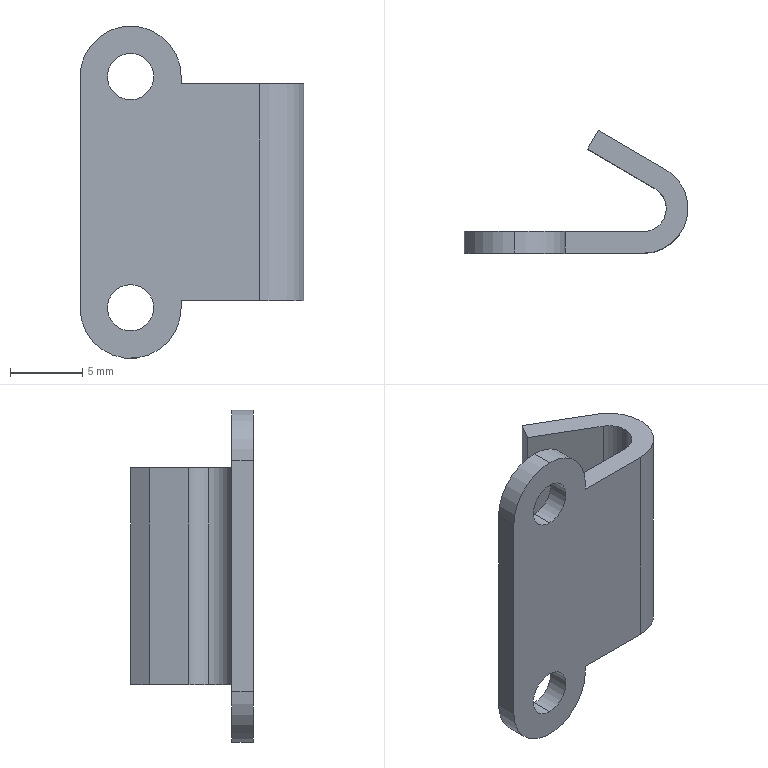Part | SolidWorks | features BaseBody 1 | 1 solid | 22 faces | box 15.5 x 8.5 x 23 mm | volume 582.779 mm3 | cylinder 11 | plane 11 | commonest cylinder face diameters 3.2 x6 7 x3 6.2 x2
STEP:
#1=CARTESIAN_POINT('',(-12.4,-3.1,8.));
#2=VERTEX_POINT('',#1);
#3=CARTESIAN_POINT('',(-8.9,-3.1,11.5));
#4=VERTEX_POINT('',#3);
#5=CARTESIAN_POINT('',(-8.9,-3.1,8.));
#6=DIRECTION('',(0.,1.,0.));
#7=DIRECTION('',(0.,0.,1.));
#8=AXIS2_PLACEMENT_3D('',#5,#6,#7);
#9=CIRCLE('',#8,3.5);
#10=EDGE_CURVE('',#2,#4,#9,.T.);
#11=ORIENTED_EDGE('',*,*,#10,.T.);
#12=CARTESIAN_POINT('',(-8.9,-1.6,11.5));
#13=VERTEX_POINT('',#12);
#14=CARTESIAN_POINT('',(-8.9,20.,11.5));
#15=DIRECTION('',(0.,1.,0.));
#16=VECTOR('',#15,1000.);
#17=LINE('',#14,#16);
#18=EDGE_CURVE('',#4,#13,#17,.T.);
#19=ORIENTED_EDGE('',*,*,#18,.T.);
#20=CARTESIAN_POINT('',(-12.4,-1.6,8.));
#21=VERTEX_POINT('',#20);
#22=CARTESIAN_POINT('',(-8.9,-1.6,8.));
#23=DIRECTION('',(0.,-1.,0.));
#24=DIRECTION('',(0.,0.,1.));
#25=AXIS2_PLACEMENT_3D('',#22,#23,#24);
#26=CIRCLE('',#25,3.5);
#27=EDGE_CURVE('',#13,#21,#26,.T.);
#28=ORIENTED_EDGE('',*,*,#27,.T.);
#29=CARTESIAN_POINT('',(-12.4,-1.6,8.));
#30=DIRECTION('',(0.,-1.,0.));
#31=VECTOR('',#30,1000.);
#32=LINE('',#29,#31);
#33=EDGE_CURVE('',#21,#2,#32,.T.);
#34=ORIENTED_EDGE('',*,*,#33,.T.);
#35=EDGE_LOOP('',(#11,#19,#28,#34));
#36=FACE_OUTER_BOUND('',#35,.T.);
#37=CARTESIAN_POINT('',(-8.9,20.,8.));
#38=DIRECTION('',(0.,1.,0.));
#39=DIRECTION('',(0.,0.,1.));
#40=AXIS2_PLACEMENT_3D('',#37,#38,#39);
#41=CYLINDRICAL_SURFACE('',#40,3.5);
#42=ADVANCED_FACE('',(#36),#41,.T.);
#43=CARTESIAN_POINT('',(-8.9,-3.1,-6.4));
#44=VERTEX_POINT('',#43);
#45=CARTESIAN_POINT('',(-8.9,-3.1,-9.6));
#46=VERTEX_POINT('',#45);
#47=CARTESIAN_POINT('',(-8.9,-3.1,-8.));
#48=DIRECTION('',(0.,-1.,0.));
#49=DIRECTION('',(0.,0.,1.));
#50=AXIS2_PLACEMENT_3D('',#47,#48,#49);
#51=CIRCLE('',#50,1.6);
#52=EDGE_CURVE('',#44,#46,#51,.T.);
#53=ORIENTED_EDGE('',*,*,#52,.T.);
#54=CARTESIAN_POINT('',(-8.9,-1.6,-9.6));
#55=VERTEX_POINT('',#54);
#56=CARTESIAN_POINT('',(-8.9,20.,-9.6));
#57=DIRECTION('',(0.,1.,0.));
#58=VECTOR('',#57,1000.);
#59=LINE('',#56,#58);
#60=EDGE_CURVE('',#46,#55,#59,.T.);
#61=ORIENTED_EDGE('',*,*,#60,.T.);
#62=CARTESIAN_POINT('',(-8.9,-1.6,-6.4));
#63=VERTEX_POINT('',#62);
#64=CARTESIAN_POINT('',(-8.9,-1.6,-8.));
#65=DIRECTION('',(0.,-1.,0.));
#66=DIRECTION('',(0.,0.,1.));
#67=AXIS2_PLACEMENT_3D('',#64,#65,#66);
#68=CIRCLE('',#67,1.6);
#69=EDGE_CURVE('',#63,#55,#68,.T.);
#70=ORIENTED_EDGE('',*,*,#69,.F.);
#71=CARTESIAN_POINT('',(-8.9,20.,-6.4));
#72=DIRECTION('',(0.,1.,0.));
#73=VECTOR('',#72,1000.);
#74=LINE('',#71,#73);
#75=EDGE_CURVE('',#44,#63,#74,.T.);
#76=ORIENTED_EDGE('',*,*,#75,.F.);
#77=EDGE_LOOP('',(#53,#61,#70,#76));
#78=FACE_OUTER_BOUND('',#77,.T.);
#79=CARTESIAN_POINT('',(-8.9,20.,-8.));
#80=DIRECTION('',(0.,1.,0.));
#81=DIRECTION('',(0.,0.,1.));
#82=AXIS2_PLACEMENT_3D('',#79,#80,#81);
#83=CYLINDRICAL_SURFACE('',#82,1.6);
#84=ADVANCED_FACE('',(#78),#83,.F.);
#85=CARTESIAN_POINT('',(-8.9,-3.1,9.6));
#86=VERTEX_POINT('',#85);
#87=CARTESIAN_POINT('',(-8.9,-3.1,6.4));
#88=VERTEX_POINT('',#87);
#89=CARTESIAN_POINT('',(-8.9,-3.1,8.));
#90=DIRECTION('',(0.,-1.,0.));
#91=DIRECTION('',(0.,0.,1.));
#92=AXIS2_PLACEMENT_3D('',#89,#90,#91);
#93=CIRCLE('',#92,1.6);
#94=EDGE_CURVE('',#86,#88,#93,.T.);
#95=ORIENTED_EDGE('',*,*,#94,.T.);
#96=CARTESIAN_POINT('',(-8.9,-1.6,6.4));
#97=VERTEX_POINT('',#96);
#98=CARTESIAN_POINT('',(-8.9,20.,6.4));
#99=DIRECTION('',(0.,1.,0.));
#100=VECTOR('',#99,1000.);
#101=LINE('',#98,#100);
#102=EDGE_CURVE('',#88,#97,#101,.T.);
#103=ORIENTED_EDGE('',*,*,#102,.T.);
#104=CARTESIAN_POINT('',(-8.9,-1.6,9.6));
#105=VERTEX_POINT('',#104);
#106=CARTESIAN_POINT('',(-8.9,-1.6,8.));
#107=DIRECTION('',(0.,-1.,0.));
#108=DIRECTION('',(0.,0.,1.));
#109=AXIS2_PLACEMENT_3D('',#106,#107,#108);
#110=CIRCLE('',#109,1.6);
#111=EDGE_CURVE('',#105,#97,#110,.T.);
#112=ORIENTED_EDGE('',*,*,#111,.F.);
#113=CARTESIAN_POINT('',(-8.9,20.,9.6));
#114=DIRECTION('',(0.,1.,0.));
#115=VECTOR('',#114,1000.);
#116=LINE('',#113,#115);
#117=EDGE_CURVE('',#86,#105,#116,.T.);
#118=ORIENTED_EDGE('',*,*,#117,.F.);
#119=EDGE_LOOP('',(#95,#103,#112,#118));
#120=FACE_OUTER_BOUND('',#119,.T.);
#121=CARTESIAN_POINT('',(-8.9,20.,8.));
#122=DIRECTION('',(0.,1.,0.));
#123=DIRECTION('',(0.,0.,1.));
#124=AXIS2_PLACEMENT_3D('',#121,#122,#123);
#125=CYLINDRICAL_SURFACE('',#124,1.6);
#126=ADVANCED_FACE('',(#120),#125,.F.);
#127=CARTESIAN_POINT('',(0.8076,1.382,-7.5));
#128=VERTEX_POINT('',#127);
#129=CARTESIAN_POINT('',(1.601,0.,-7.5));
#130=VERTEX_POINT('',#129);
#131=CARTESIAN_POINT('',(0.0007268,0.,-7.5));
#132=DIRECTION('',(0.,0.,-1.));
#133=DIRECTION('',(1.,0.,0.));
#134=AXIS2_PLACEMENT_3D('',#131,#132,#133);
#135=CIRCLE('',#134,1.6);
#136=EDGE_CURVE('',#128,#130,#135,.T.);
#137=ORIENTED_EDGE('',*,*,#136,.T.);
#138=CARTESIAN_POINT('',(1.601,0.,7.5));
#139=VERTEX_POINT('',#138);
#140=CARTESIAN_POINT('',(1.601,0.,20.));
#141=DIRECTION('',(0.,0.,1.));
#142=VECTOR('',#141,1000.);
#143=LINE('',#140,#142);
#144=EDGE_CURVE('',#130,#139,#143,.T.);
#145=ORIENTED_EDGE('',*,*,#144,.T.);
#146=CARTESIAN_POINT('',(0.8076,1.382,7.5));
#147=VERTEX_POINT('',#146);
#148=CARTESIAN_POINT('',(0.0007268,0.,7.5));
#149=DIRECTION('',(0.,0.,1.));
#150=DIRECTION('',(1.,0.,0.));
#151=AXIS2_PLACEMENT_3D('',#148,#149,#150);
#152=CIRCLE('',#151,1.6);
#153=EDGE_CURVE('',#139,#147,#152,.T.);
#154=ORIENTED_EDGE('',*,*,#153,.T.);
#155=CARTESIAN_POINT('',(0.8076,1.382,20.));
#156=DIRECTION('',(0.,0.,1.));
#157=VECTOR('',#156,1000.);
#158=LINE('',#155,#157);
#159=EDGE_CURVE('',#128,#147,#158,.T.);
#160=ORIENTED_EDGE('',*,*,#159,.F.);
#161=EDGE_LOOP('',(#137,#145,#154,#160));
#162=FACE_OUTER_BOUND('',#161,.T.);
#163=CARTESIAN_POINT('',(0.0007268,0.,20.));
#164=DIRECTION('',(0.,0.,1.));
#165=DIRECTION('',(1.,0.,0.));
#166=AXIS2_PLACEMENT_3D('',#163,#164,#165);
#167=CYLINDRICAL_SURFACE('',#166,1.6);
#168=ADVANCED_FACE('',(#162),#167,.F.);
#169=CARTESIAN_POINT('',(-3.856,4.105,-7.5));
#170=VERTEX_POINT('',#169);
#171=CARTESIAN_POINT('',(-3.1,5.4,-7.5));
#172=VERTEX_POINT('',#171);
#173=CARTESIAN_POINT('',(-3.1,5.4,-7.5));
#174=DIRECTION('',(0.5042,0.8636,0.));
#175=VECTOR('',#174,1000.);
#176=LINE('',#173,#175);
#177=EDGE_CURVE('',#170,#172,#176,.T.);
#178=ORIENTED_EDGE('',*,*,#177,.F.);
#179=CARTESIAN_POINT('',(-3.856,4.105,7.5));
#180=VERTEX_POINT('',#179);
#181=CARTESIAN_POINT('',(-3.856,4.105,20.));
#182=DIRECTION('',(0.,0.,1.));
#183=VECTOR('',#182,1000.);
#184=LINE('',#181,#183);
#185=EDGE_CURVE('',#170,#180,#184,.T.);
#186=ORIENTED_EDGE('',*,*,#185,.T.);
#187=CARTESIAN_POINT('',(-3.1,5.4,7.5));
#188=VERTEX_POINT('',#187);
#189=CARTESIAN_POINT('',(-3.1,5.4,7.5));
#190=DIRECTION('',(-0.5042,-0.8636,0.));
#191=VECTOR('',#190,1000.);
#192=LINE('',#189,#191);
#193=EDGE_CURVE('',#188,#180,#192,.T.);
#194=ORIENTED_EDGE('',*,*,#193,.F.);
#195=CARTESIAN_POINT('',(-3.1,5.4,20.));
#196=DIRECTION('',(0.,0.,-1.));
#197=VECTOR('',#196,1000.);
#198=LINE('',#195,#197);
#199=EDGE_CURVE('',#188,#172,#198,.T.);
#200=ORIENTED_EDGE('',*,*,#199,.T.);
#201=EDGE_LOOP('',(#178,#186,#194,#200));
#202=FACE_OUTER_BOUND('',#201,.T.);
#203=CARTESIAN_POINT('',(-3.1,5.4,20.));
#204=DIRECTION('',(0.8636,-0.5042,0.));
#205=DIRECTION('',(0.,0.,-1.));
#206=AXIS2_PLACEMENT_3D('',#203,#204,#205);
#207=PLANE('',#206);
#208=ADVANCED_FACE('',(#202),#207,.F.);
#209=CARTESIAN_POINT('',(-5.4,-1.6,7.5));
#210=VERTEX_POINT('',#209);
#211=CARTESIAN_POINT('',(-5.4,-1.6,8.));
#212=VERTEX_POINT('',#211);
#213=CARTESIAN_POINT('',(-5.4,-1.6,20.));
#214=DIRECTION('',(0.,0.,1.));
#215=VECTOR('',#214,1000.);
#216=LINE('',#213,#215);
#217=EDGE_CURVE('',#210,#212,#216,.T.);
#218=ORIENTED_EDGE('',*,*,#217,.T.);
#219=CARTESIAN_POINT('',(-5.4,-3.1,8.));
#220=VERTEX_POINT('',#219);
#221=CARTESIAN_POINT('',(-5.4,20.,8.));
#222=DIRECTION('',(0.,1.,0.));
#223=VECTOR('',#222,1000.);
#224=LINE('',#221,#223);
#225=EDGE_CURVE('',#220,#212,#224,.T.);
#226=ORIENTED_EDGE('',*,*,#225,.F.);
#227=CARTESIAN_POINT('',(-5.4,-3.1,7.5));
#228=VERTEX_POINT('',#227);
#229=CARTESIAN_POINT('',(-5.4,-3.1,8.));
#230=DIRECTION('',(0.,0.,1.));
#231=VECTOR('',#230,1000.);
#232=LINE('',#229,#231);
#233=EDGE_CURVE('',#228,#220,#232,.T.);
#234=ORIENTED_EDGE('',*,*,#233,.F.);
#235=CARTESIAN_POINT('',(-5.4,20.,7.5));
#236=DIRECTION('',(0.,1.,0.));
#237=VECTOR('',#236,1000.);
#238=LINE('',#235,#237);
#239=EDGE_CURVE('',#228,#210,#238,.T.);
#240=ORIENTED_EDGE('',*,*,#239,.T.);
#241=EDGE_LOOP('',(#218,#226,#234,#240));
#242=FACE_OUTER_BOUND('',#241,.T.);
#243=CARTESIAN_POINT('',(-5.4,20.,8.));
#244=DIRECTION('',(-1.,0.,0.));
#245=DIRECTION('',(0.,0.,1.));
#246=AXIS2_PLACEMENT_3D('',#243,#244,#245);
#247=PLANE('',#246);
#248=ADVANCED_FACE('',(#242),#247,.F.);
#249=CARTESIAN_POINT('',(3.1,-0.06933,-7.5));
#250=VERTEX_POINT('',#249);
#251=CARTESIAN_POINT('',(3.1,-0.06933,7.5));
#252=VERTEX_POINT('',#251);
#253=CARTESIAN_POINT('',(3.1,-0.06933,20.));
#254=DIRECTION('',(0.,0.,1.));
#255=VECTOR('',#254,1000.);
#256=LINE('',#253,#255);
#257=EDGE_CURVE('',#250,#252,#256,.T.);
#258=ORIENTED_EDGE('',*,*,#257,.F.);
#259=CARTESIAN_POINT('',(3.1,0.06933,-7.5));
#260=VERTEX_POINT('',#259);
#261=CARTESIAN_POINT('',(3.1,20.,-7.5));
#262=DIRECTION('',(0.,-1.,0.));
#263=VECTOR('',#262,1000.);
#264=LINE('',#261,#263);
#265=EDGE_CURVE('',#260,#250,#264,.T.);
#266=ORIENTED_EDGE('',*,*,#265,.F.);
#267=CARTESIAN_POINT('',(3.1,0.06933,7.5));
#268=VERTEX_POINT('',#267);
#269=CARTESIAN_POINT('',(3.1,0.06933,20.));
#270=DIRECTION('',(0.,0.,-1.));
#271=VECTOR('',#270,1000.);
#272=LINE('',#269,#271);
#273=EDGE_CURVE('',#268,#260,#272,.T.);
#274=ORIENTED_EDGE('',*,*,#273,.F.);
#275=CARTESIAN_POINT('',(3.1,20.,7.5));
#276=DIRECTION('',(0.,-1.,0.));
#277=VECTOR('',#276,1000.);
#278=LINE('',#275,#277);
#279=EDGE_CURVE('',#268,#252,#278,.T.);
#280=ORIENTED_EDGE('',*,*,#279,.T.);
#281=EDGE_LOOP('',(#258,#266,#274,#280));
#282=FACE_OUTER_BOUND('',#281,.T.);
#283=CARTESIAN_POINT('',(3.1,20.,7.5));
#284=DIRECTION('',(-1.,0.,0.));
#285=DIRECTION('',(0.,0.,1.));
#286=AXIS2_PLACEMENT_3D('',#283,#284,#285);
#287=PLANE('',#286);
#288=ADVANCED_FACE('',(#282),#287,.F.);
#289=CARTESIAN_POINT('',(1.564,2.677,-7.5));
#290=VERTEX_POINT('',#289);
#291=CARTESIAN_POINT('',(1.564,2.677,7.5));
#292=VERTEX_POINT('',#291);
#293=CARTESIAN_POINT('',(1.564,2.677,20.));
#294=DIRECTION('',(0.,0.,1.));
#295=VECTOR('',#294,1000.);
#296=LINE('',#293,#295);
#297=EDGE_CURVE('',#290,#292,#296,.T.);
#298=ORIENTED_EDGE('',*,*,#297,.T.);
#299=CARTESIAN_POINT('',(0.0007754,0.,7.5));
#300=DIRECTION('',(0.,0.,-1.));
#301=DIRECTION('',(1.,0.,0.));
#302=AXIS2_PLACEMENT_3D('',#299,#300,#301);
#303=CIRCLE('',#302,3.1);
#304=EDGE_CURVE('',#292,#268,#303,.T.);
#305=ORIENTED_EDGE('',*,*,#304,.T.);
#306=ORIENTED_EDGE('',*,*,#273,.T.);
#307=CARTESIAN_POINT('',(0.0007754,0.,-7.5));
#308=DIRECTION('',(0.,0.,1.));
#309=DIRECTION('',(1.,0.,0.));
#310=AXIS2_PLACEMENT_3D('',#307,#308,#309);
#311=CIRCLE('',#310,3.1);
#312=EDGE_CURVE('',#260,#290,#311,.T.);
#313=ORIENTED_EDGE('',*,*,#312,.T.);
#314=EDGE_LOOP('',(#298,#305,#306,#313));
#315=FACE_OUTER_BOUND('',#314,.T.);
#316=CARTESIAN_POINT('',(0.0007754,0.,20.));
#317=DIRECTION('',(0.,0.,1.));
#318=DIRECTION('',(1.,0.,0.));
#319=AXIS2_PLACEMENT_3D('',#316,#317,#318);
#320=CYLINDRICAL_SURFACE('',#319,3.1);
#321=ADVANCED_FACE('',(#315),#320,.T.);
#322=CARTESIAN_POINT('',(1.564,2.677,-7.5));
#323=DIRECTION('',(-0.8636,0.5042,0.));
#324=VECTOR('',#323,1000.);
#325=LINE('',#322,#324);
#326=EDGE_CURVE('',#290,#172,#325,.T.);
#327=ORIENTED_EDGE('',*,*,#326,.T.);
#328=ORIENTED_EDGE('',*,*,#199,.F.);
#329=CARTESIAN_POINT('',(-3.1,5.4,7.5));
#330=DIRECTION('',(0.8636,-0.5042,0.));
#331=VECTOR('',#330,1000.);
#332=LINE('',#329,#331);
#333=EDGE_CURVE('',#188,#292,#332,.T.);
#334=ORIENTED_EDGE('',*,*,#333,.T.);
#335=ORIENTED_EDGE('',*,*,#297,.F.);
#336=EDGE_LOOP('',(#327,#328,#334,#335));
#337=FACE_OUTER_BOUND('',#336,.T.);
#338=CARTESIAN_POINT('',(1.564,2.677,20.));
#339=DIRECTION('',(-0.5042,-0.8636,0.));
#340=DIRECTION('',(-0.8636,0.5042,0.));
#341=AXIS2_PLACEMENT_3D('',#338,#339,#340);
#342=PLANE('',#341);
#343=ADVANCED_FACE('',(#337),#342,.F.);
#344=CARTESIAN_POINT('',(-3.856,4.105,-7.5));
#345=DIRECTION('',(0.8635,-0.5043,0.));
#346=VECTOR('',#345,1000.);
#347=LINE('',#344,#346);
#348=EDGE_CURVE('',#170,#128,#347,.T.);
#349=ORIENTED_EDGE('',*,*,#348,.T.);
#350=ORIENTED_EDGE('',*,*,#159,.T.);
#351=CARTESIAN_POINT('',(0.8076,1.382,7.5));
#352=DIRECTION('',(-0.8635,0.5043,0.));
#353=VECTOR('',#352,1000.);
#354=LINE('',#351,#353);
#355=EDGE_CURVE('',#147,#180,#354,.T.);
#356=ORIENTED_EDGE('',*,*,#355,.T.);
#357=ORIENTED_EDGE('',*,*,#185,.F.);
#358=EDGE_LOOP('',(#349,#350,#356,#357));
#359=FACE_OUTER_BOUND('',#358,.T.);
#360=CARTESIAN_POINT('',(-3.856,4.105,20.));
#361=DIRECTION('',(0.5043,0.8635,0.));
#362=DIRECTION('',(0.,0.,-1.));
#363=AXIS2_PLACEMENT_3D('',#360,#361,#362);
#364=PLANE('',#363);
#365=ADVANCED_FACE('',(#359),#364,.F.);
#366=CARTESIAN_POINT('',(-5.4,-1.6,-8.));
#367=VERTEX_POINT('',#366);
#368=CARTESIAN_POINT('',(-5.4,-1.6,-7.5));
#369=VERTEX_POINT('',#368);
#370=CARTESIAN_POINT('',(-5.4,-1.6,20.));
#371=DIRECTION('',(0.,0.,1.));
#372=VECTOR('',#371,1000.);
#373=LINE('',#370,#372);
#374=EDGE_CURVE('',#367,#369,#373,.T.);
#375=ORIENTED_EDGE('',*,*,#374,.T.);
#376=CARTESIAN_POINT('',(-5.4,-3.1,-7.5));
#377=VERTEX_POINT('',#376);
#378=CARTESIAN_POINT('',(-5.4,20.,-7.5));
#379=DIRECTION('',(0.,-1.,0.));
#380=VECTOR('',#379,1000.);
#381=LINE('',#378,#380);
#382=EDGE_CURVE('',#369,#377,#381,.T.);
#383=ORIENTED_EDGE('',*,*,#382,.T.);
#384=CARTESIAN_POINT('',(-5.4,-3.1,-8.));
#385=VERTEX_POINT('',#384);
#386=CARTESIAN_POINT('',(-5.4,-3.1,-7.5));
#387=DIRECTION('',(0.,0.,1.));
#388=VECTOR('',#387,1000.);
#389=LINE('',#386,#388);
#390=EDGE_CURVE('',#385,#377,#389,.T.);
#391=ORIENTED_EDGE('',*,*,#390,.F.);
#392=CARTESIAN_POINT('',(-5.4,20.,-8.));
#393=DIRECTION('',(0.,-1.,0.));
#394=VECTOR('',#393,1000.);
#395=LINE('',#392,#394);
#396=EDGE_CURVE('',#367,#385,#395,.T.);
#397=ORIENTED_EDGE('',*,*,#396,.F.);
#398=EDGE_LOOP('',(#375,#383,#391,#397));
#399=FACE_OUTER_BOUND('',#398,.T.);
#400=CARTESIAN_POINT('',(-5.4,20.,-7.5));
#401=DIRECTION('',(-1.,0.,0.));
#402=DIRECTION('',(0.,0.,1.));
#403=AXIS2_PLACEMENT_3D('',#400,#401,#402);
#404=PLANE('',#403);
#405=ADVANCED_FACE('',(#399),#404,.F.);
#406=ORIENTED_EDGE('',*,*,#111,.T.);
#407=CARTESIAN_POINT('',(-8.9,-1.6,8.));
#408=DIRECTION('',(0.,-1.,0.));
#409=DIRECTION('',(0.,0.,1.));
#410=AXIS2_PLACEMENT_3D('',#407,#408,#409);
#411=CIRCLE('',#410,1.6);
#412=EDGE_CURVE('',#97,#105,#411,.T.);
#413=ORIENTED_EDGE('',*,*,#412,.T.);
#414=EDGE_LOOP('',(#406,#413));
#415=FACE_BOUND('',#414,.T.);
#416=ORIENTED_EDGE('',*,*,#69,.T.);
#417=CARTESIAN_POINT('',(-8.9,-1.6,-8.));
#418=DIRECTION('',(0.,-1.,0.));
#419=DIRECTION('',(0.,0.,1.));
#420=AXIS2_PLACEMENT_3D('',#417,#418,#419);
#421=CIRCLE('',#420,1.6);
#422=EDGE_CURVE('',#55,#63,#421,.T.);
#423=ORIENTED_EDGE('',*,*,#422,.T.);
#424=EDGE_LOOP('',(#416,#423));
#425=FACE_BOUND('',#424,.T.);
#426=CARTESIAN_POINT('',(-12.4,-1.6,-8.));
#427=VERTEX_POINT('',#426);
#428=CARTESIAN_POINT('',(-8.9,-1.6,-8.));
#429=DIRECTION('',(0.,-1.,0.));
#430=DIRECTION('',(0.,0.,1.));
#431=AXIS2_PLACEMENT_3D('',#428,#429,#430);
#432=CIRCLE('',#431,3.5);
#433=EDGE_CURVE('',#427,#367,#432,.T.);
#434=ORIENTED_EDGE('',*,*,#433,.F.);
#435=CARTESIAN_POINT('',(-12.4,-1.6,20.));
#436=DIRECTION('',(0.,0.,1.));
#437=VECTOR('',#436,1000.);
#438=LINE('',#435,#437);
#439=EDGE_CURVE('',#427,#21,#438,.T.);
#440=ORIENTED_EDGE('',*,*,#439,.T.);
#441=ORIENTED_EDGE('',*,*,#27,.F.);
#442=CARTESIAN_POINT('',(-8.9,-1.6,8.));
#443=DIRECTION('',(0.,-1.,0.));
#444=DIRECTION('',(0.,0.,1.));
#445=AXIS2_PLACEMENT_3D('',#442,#443,#444);
#446=CIRCLE('',#445,3.5);
#447=EDGE_CURVE('',#212,#13,#446,.T.);
#448=ORIENTED_EDGE('',*,*,#447,.F.);
#449=ORIENTED_EDGE('',*,*,#217,.F.);
#450=CARTESIAN_POINT('',(0.0007271,-1.6,7.5));
#451=VERTEX_POINT('',#450);
#452=CARTESIAN_POINT('',(-5.4,-1.6,7.5));
#453=DIRECTION('',(1.,0.,0.));
#454=VECTOR('',#453,1000.);
#455=LINE('',#452,#454);
#456=EDGE_CURVE('',#210,#451,#455,.T.);
#457=ORIENTED_EDGE('',*,*,#456,.T.);
#458=CARTESIAN_POINT('',(0.0007271,-1.6,-7.5));
#459=VERTEX_POINT('',#458);
#460=CARTESIAN_POINT('',(0.0007274,-1.6,20.));
#461=DIRECTION('',(0.,0.,1.));
#462=VECTOR('',#461,1000.);
#463=LINE('',#460,#462);
#464=EDGE_CURVE('',#459,#451,#463,.T.);
#465=ORIENTED_EDGE('',*,*,#464,.F.);
#466=CARTESIAN_POINT('',(3.1,-1.6,-7.5));
#467=DIRECTION('',(-1.,0.,0.));
#468=VECTOR('',#467,1000.);
#469=LINE('',#466,#468);
#470=EDGE_CURVE('',#459,#369,#469,.T.);
#471=ORIENTED_EDGE('',*,*,#470,.T.);
#472=ORIENTED_EDGE('',*,*,#374,.F.);
#473=EDGE_LOOP('',(#434,#440,#441,#448,#449,#457,#465,#471,#472));
#474=FACE_OUTER_BOUND('',#473,.T.);
#475=CARTESIAN_POINT('',(0.0007274,-1.6,20.));
#476=DIRECTION('',(0.,-1.,0.));
#477=DIRECTION('',(0.,0.,-1.));
#478=AXIS2_PLACEMENT_3D('',#475,#476,#477);
#479=PLANE('',#478);
#480=ADVANCED_FACE('',(#415,#425,#474),#479,.F.);
#481=ORIENTED_EDGE('',*,*,#279,.F.);
#482=ORIENTED_EDGE('',*,*,#304,.F.);
#483=ORIENTED_EDGE('',*,*,#333,.F.);
#484=ORIENTED_EDGE('',*,*,#193,.T.);
#485=ORIENTED_EDGE('',*,*,#355,.F.);
#486=ORIENTED_EDGE('',*,*,#153,.F.);
#487=CARTESIAN_POINT('',(0.0007268,0.,7.5));
#488=DIRECTION('',(0.,0.,1.));
#489=DIRECTION('',(1.,0.,0.));
#490=AXIS2_PLACEMENT_3D('',#487,#488,#489);
#491=CIRCLE('',#490,1.6);
#492=EDGE_CURVE('',#451,#139,#491,.T.);
#493=ORIENTED_EDGE('',*,*,#492,.F.);
#494=ORIENTED_EDGE('',*,*,#456,.F.);
#495=ORIENTED_EDGE('',*,*,#239,.F.);
#496=CARTESIAN_POINT('',(0.0007755,-3.1,7.5));
#497=VERTEX_POINT('',#496);
#498=CARTESIAN_POINT('',(-12.4,-3.1,7.5));
#499=DIRECTION('',(1.,0.,0.));
#500=VECTOR('',#499,1000.);
#501=LINE('',#498,#500);
#502=EDGE_CURVE('',#228,#497,#501,.T.);
#503=ORIENTED_EDGE('',*,*,#502,.T.);
#504=CARTESIAN_POINT('',(0.0007754,0.,7.5));
#505=DIRECTION('',(0.,0.,-1.));
#506=DIRECTION('',(1.,0.,0.));
#507=AXIS2_PLACEMENT_3D('',#504,#505,#506);
#508=CIRCLE('',#507,3.1);
#509=EDGE_CURVE('',#252,#497,#508,.T.);
#510=ORIENTED_EDGE('',*,*,#509,.F.);
#511=EDGE_LOOP('',(#481,#482,#483,#484,#485,#486,#493,#494,#495,#503,#510));
#512=FACE_OUTER_BOUND('',#511,.T.);
#513=CARTESIAN_POINT('',(-5.4,20.,7.5));
#514=DIRECTION('',(0.,0.,-1.));
#515=DIRECTION('',(0.,-1.,0.));
#516=AXIS2_PLACEMENT_3D('',#513,#514,#515);
#517=PLANE('',#516);
#518=ADVANCED_FACE('',(#512),#517,.F.);
#519=ORIENTED_EDGE('',*,*,#257,.T.);
#520=ORIENTED_EDGE('',*,*,#509,.T.);
#521=CARTESIAN_POINT('',(0.0007755,-3.1,-7.5));
#522=VERTEX_POINT('',#521);
#523=CARTESIAN_POINT('',(0.0007756,-3.1,20.));
#524=DIRECTION('',(0.,0.,-1.));
#525=VECTOR('',#524,1000.);
#526=LINE('',#523,#525);
#527=EDGE_CURVE('',#497,#522,#526,.T.);
#528=ORIENTED_EDGE('',*,*,#527,.T.);
#529=CARTESIAN_POINT('',(0.0007754,0.,-7.5));
#530=DIRECTION('',(0.,0.,1.));
#531=DIRECTION('',(1.,0.,0.));
#532=AXIS2_PLACEMENT_3D('',#529,#530,#531);
#533=CIRCLE('',#532,3.1);
#534=EDGE_CURVE('',#522,#250,#533,.T.);
#535=ORIENTED_EDGE('',*,*,#534,.T.);
#536=EDGE_LOOP('',(#519,#520,#528,#535));
#537=FACE_OUTER_BOUND('',#536,.T.);
#538=CARTESIAN_POINT('',(0.0007754,0.,20.));
#539=DIRECTION('',(0.,0.,1.));
#540=DIRECTION('',(1.,0.,0.));
#541=AXIS2_PLACEMENT_3D('',#538,#539,#540);
#542=CYLINDRICAL_SURFACE('',#541,3.1);
#543=ADVANCED_FACE('',(#537),#542,.T.);
#544=ORIENTED_EDGE('',*,*,#470,.F.);
#545=CARTESIAN_POINT('',(0.0007268,0.,-7.5));
#546=DIRECTION('',(0.,0.,-1.));
#547=DIRECTION('',(1.,0.,0.));
#548=AXIS2_PLACEMENT_3D('',#545,#546,#547);
#549=CIRCLE('',#548,1.6);
#550=EDGE_CURVE('',#130,#459,#549,.T.);
#551=ORIENTED_EDGE('',*,*,#550,.F.);
#552=ORIENTED_EDGE('',*,*,#136,.F.);
#553=ORIENTED_EDGE('',*,*,#348,.F.);
#554=ORIENTED_EDGE('',*,*,#177,.T.);
#555=ORIENTED_EDGE('',*,*,#326,.F.);
#556=ORIENTED_EDGE('',*,*,#312,.F.);
#557=ORIENTED_EDGE('',*,*,#265,.T.);
#558=ORIENTED_EDGE('',*,*,#534,.F.);
#559=CARTESIAN_POINT('',(-12.4,-3.1,-7.5));
#560=DIRECTION('',(-1.,0.,0.));
#561=VECTOR('',#560,1000.);
#562=LINE('',#559,#561);
#563=EDGE_CURVE('',#522,#377,#562,.T.);
#564=ORIENTED_EDGE('',*,*,#563,.T.);
#565=ORIENTED_EDGE('',*,*,#382,.F.);
#566=EDGE_LOOP('',(#544,#551,#552,#553,#554,#555,#556,#557,#558,#564,#565));
#567=FACE_OUTER_BOUND('',#566,.T.);
#568=CARTESIAN_POINT('',(3.1,20.,-7.5));
#569=DIRECTION('',(0.,0.,1.));
#570=DIRECTION('',(1.,0.,0.));
#571=AXIS2_PLACEMENT_3D('',#568,#569,#570);
#572=PLANE('',#571);
#573=ADVANCED_FACE('',(#567),#572,.F.);
#574=ORIENTED_EDGE('',*,*,#396,.T.);
#575=CARTESIAN_POINT('',(-12.4,-3.1,-8.));
#576=VERTEX_POINT('',#575);
#577=CARTESIAN_POINT('',(-8.9,-3.1,-8.));
#578=DIRECTION('',(0.,1.,0.));
#579=DIRECTION('',(0.,0.,1.));
#580=AXIS2_PLACEMENT_3D('',#577,#578,#579);
#581=CIRCLE('',#580,3.5);
#582=EDGE_CURVE('',#385,#576,#581,.T.);
#583=ORIENTED_EDGE('',*,*,#582,.T.);
#584=CARTESIAN_POINT('',(-12.4,-1.6,-8.));
#585=DIRECTION('',(0.,1.,0.));
#586=VECTOR('',#585,1000.);
#587=LINE('',#584,#586);
#588=EDGE_CURVE('',#576,#427,#587,.T.);
#589=ORIENTED_EDGE('',*,*,#588,.T.);
#590=ORIENTED_EDGE('',*,*,#433,.T.);
#591=EDGE_LOOP('',(#574,#583,#589,#590));
#592=FACE_OUTER_BOUND('',#591,.T.);
#593=CARTESIAN_POINT('',(-8.9,20.,-8.));
#594=DIRECTION('',(0.,1.,0.));
#595=DIRECTION('',(0.,0.,1.));
#596=AXIS2_PLACEMENT_3D('',#593,#594,#595);
#597=CYLINDRICAL_SURFACE('',#596,3.5);
#598=ADVANCED_FACE('',(#592),#597,.T.);
#599=CARTESIAN_POINT('',(-12.4,-3.1,20.));
#600=DIRECTION('',(0.,0.,1.));
#601=VECTOR('',#600,1000.);
#602=LINE('',#599,#601);
#603=EDGE_CURVE('',#576,#2,#602,.T.);
#604=ORIENTED_EDGE('',*,*,#603,.T.);
#605=ORIENTED_EDGE('',*,*,#33,.F.);
#606=ORIENTED_EDGE('',*,*,#439,.F.);
#607=ORIENTED_EDGE('',*,*,#588,.F.);
#608=EDGE_LOOP('',(#604,#605,#606,#607));
#609=FACE_OUTER_BOUND('',#608,.T.);
#610=CARTESIAN_POINT('',(-12.4,-1.6,20.));
#611=DIRECTION('',(1.,0.,0.));
#612=DIRECTION('',(0.,1.,0.));
#613=AXIS2_PLACEMENT_3D('',#610,#611,#612);
#614=PLANE('',#613);
#615=ADVANCED_FACE('',(#609),#614,.F.);
#616=ORIENTED_EDGE('',*,*,#94,.F.);
#617=CARTESIAN_POINT('',(-8.9,-3.1,8.));
#618=DIRECTION('',(0.,-1.,0.));
#619=DIRECTION('',(0.,0.,1.));
#620=AXIS2_PLACEMENT_3D('',#617,#618,#619);
#621=CIRCLE('',#620,1.6);
#622=EDGE_CURVE('',#88,#86,#621,.T.);
#623=ORIENTED_EDGE('',*,*,#622,.F.);
#624=EDGE_LOOP('',(#616,#623));
#625=FACE_BOUND('',#624,.T.);
#626=ORIENTED_EDGE('',*,*,#52,.F.);
#627=CARTESIAN_POINT('',(-8.9,-3.1,-8.));
#628=DIRECTION('',(0.,-1.,0.));
#629=DIRECTION('',(0.,0.,1.));
#630=AXIS2_PLACEMENT_3D('',#627,#628,#629);
#631=CIRCLE('',#630,1.6);
#632=EDGE_CURVE('',#46,#44,#631,.T.);
#633=ORIENTED_EDGE('',*,*,#632,.F.);
#634=EDGE_LOOP('',(#626,#633));
#635=FACE_BOUND('',#634,.T.);
#636=ORIENTED_EDGE('',*,*,#582,.F.);
#637=ORIENTED_EDGE('',*,*,#390,.T.);
#638=ORIENTED_EDGE('',*,*,#563,.F.);
#639=ORIENTED_EDGE('',*,*,#527,.F.);
#640=ORIENTED_EDGE('',*,*,#502,.F.);
#641=ORIENTED_EDGE('',*,*,#233,.T.);
#642=CARTESIAN_POINT('',(-8.9,-3.1,8.));
#643=DIRECTION('',(0.,1.,0.));
#644=DIRECTION('',(0.,0.,1.));
#645=AXIS2_PLACEMENT_3D('',#642,#643,#644);
#646=CIRCLE('',#645,3.5);
#647=EDGE_CURVE('',#4,#220,#646,.T.);
#648=ORIENTED_EDGE('',*,*,#647,.F.);
#649=ORIENTED_EDGE('',*,*,#10,.F.);
#650=ORIENTED_EDGE('',*,*,#603,.F.);
#651=EDGE_LOOP('',(#636,#637,#638,#639,#640,#641,#648,#649,#650));
#652=FACE_OUTER_BOUND('',#651,.T.);
#653=CARTESIAN_POINT('',(-12.4,-3.1,20.));
#654=DIRECTION('',(0.,1.,0.));
#655=DIRECTION('',(1.,0.,0.));
#656=AXIS2_PLACEMENT_3D('',#653,#654,#655);
#657=PLANE('',#656);
#658=ADVANCED_FACE('',(#625,#635,#652),#657,.F.);
#659=ORIENTED_EDGE('',*,*,#144,.F.);
#660=ORIENTED_EDGE('',*,*,#550,.T.);
#661=ORIENTED_EDGE('',*,*,#464,.T.);
#662=ORIENTED_EDGE('',*,*,#492,.T.);
#663=EDGE_LOOP('',(#659,#660,#661,#662));
#664=FACE_OUTER_BOUND('',#663,.T.);
#665=CARTESIAN_POINT('',(0.0007268,0.,20.));
#666=DIRECTION('',(0.,0.,1.));
#667=DIRECTION('',(1.,0.,0.));
#668=AXIS2_PLACEMENT_3D('',#665,#666,#667);
#669=CYLINDRICAL_SURFACE('',#668,1.6);
#670=ADVANCED_FACE('',(#664),#669,.F.);
#671=ORIENTED_EDGE('',*,*,#102,.F.);
#672=ORIENTED_EDGE('',*,*,#622,.T.);
#673=ORIENTED_EDGE('',*,*,#117,.T.);
#674=ORIENTED_EDGE('',*,*,#412,.F.);
#675=EDGE_LOOP('',(#671,#672,#673,#674));
#676=FACE_OUTER_BOUND('',#675,.T.);
#677=CARTESIAN_POINT('',(-8.9,20.,8.));
#678=DIRECTION('',(0.,1.,0.));
#679=DIRECTION('',(0.,0.,1.));
#680=AXIS2_PLACEMENT_3D('',#677,#678,#679);
#681=CYLINDRICAL_SURFACE('',#680,1.6);
#682=ADVANCED_FACE('',(#676),#681,.F.);
#683=ORIENTED_EDGE('',*,*,#60,.F.);
#684=ORIENTED_EDGE('',*,*,#632,.T.);
#685=ORIENTED_EDGE('',*,*,#75,.T.);
#686=ORIENTED_EDGE('',*,*,#422,.F.);
#687=EDGE_LOOP('',(#683,#684,#685,#686));
#688=FACE_OUTER_BOUND('',#687,.T.);
#689=CARTESIAN_POINT('',(-8.9,20.,-8.));
#690=DIRECTION('',(0.,1.,0.));
#691=DIRECTION('',(0.,0.,1.));
#692=AXIS2_PLACEMENT_3D('',#689,#690,#691);
#693=CYLINDRICAL_SURFACE('',#692,1.6);
#694=ADVANCED_FACE('',(#688),#693,.F.);
#695=ORIENTED_EDGE('',*,*,#18,.F.);
#696=ORIENTED_EDGE('',*,*,#647,.T.);
#697=ORIENTED_EDGE('',*,*,#225,.T.);
#698=ORIENTED_EDGE('',*,*,#447,.T.);
#699=EDGE_LOOP('',(#695,#696,#697,#698));
#700=FACE_OUTER_BOUND('',#699,.T.);
#701=CARTESIAN_POINT('',(-8.9,20.,8.));
#702=DIRECTION('',(0.,1.,0.));
#703=DIRECTION('',(0.,0.,1.));
#704=AXIS2_PLACEMENT_3D('',#701,#702,#703);
#705=CYLINDRICAL_SURFACE('',#704,3.5);
#706=ADVANCED_FACE('',(#700),#705,.T.);
#707=CLOSED_SHELL('',(#42,#84,#126,#168,#208,#248,#288,#321,#343,#365,#405,#480,#518,#543,#573,#598,#615,#658,#670,#682,#694,#706));
#708=MANIFOLD_SOLID_BREP('',#707);
#709=CARTESIAN_POINT('',(0.,0.,0.));
#710=DIRECTION('',(0.,0.,1.));
#711=DIRECTION('',(1.,0.,0.));
#712=AXIS2_PLACEMENT_3D('',#709,#710,#711);
#713=(LENGTH_UNIT()NAMED_UNIT(*)SI_UNIT(.MILLI.,.METRE.));
#714=UNCERTAINTY_MEASURE_WITH_UNIT(LENGTH_MEASURE(0.00001),#713,'','');
#715=(NAMED_UNIT(*)PLANE_ANGLE_UNIT()SI_UNIT($,.RADIAN.));
#716=(NAMED_UNIT(*)SI_UNIT($,.STERADIAN.)SOLID_ANGLE_UNIT());
#717=(GEOMETRIC_REPRESENTATION_CONTEXT(3)GLOBAL_UNCERTAINTY_ASSIGNED_CONTEXT((#714))GLOBAL_UNIT_ASSIGNED_CONTEXT((#713,#715,#716))REPRESENTATION_CONTEXT('',''));
#718=ADVANCED_BREP_SHAPE_REPRESENTATION('',(#708,#712),#717);